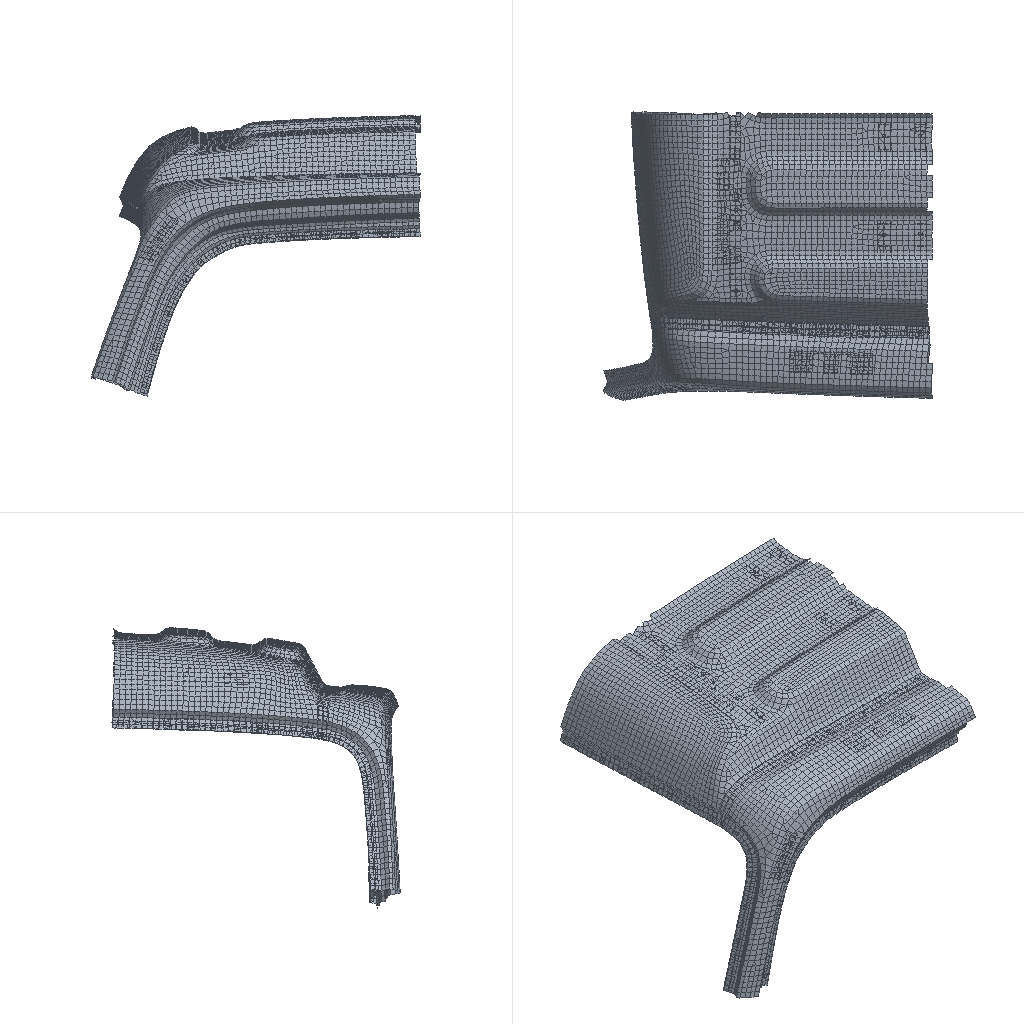Simulation study | nastran
Set-up summary:
category,name,step,type,value,unit,region
solver,nx_nastran
units,not stated in the deck,,not stated
analysis,deck,,static,static
analysis,solution,,SOL,101
load_step,SUBCASE 2,2,SUBCASE,SPC=2 LOAD=3
load_step,SUBCASE 3,3,SUBCASE,SPC=2 LOAD=4
load_step,SUBCASE 4,4,SUBCASE,SPC=2 LOAD=5
load_step,requested,,,3
mesh,nodes,,,9383
mesh,elements,,,8376
element_type,CHEXA,,unverified,79
element_type,CQUAD4,,shell,8105
element_type,CTRIA3,,shell,271
load,load commands in deck,,count,3
bc,support commands in deck,,count,307
check,setup vs results,,match,"every grid point's frame and coordinates and every element id; grid points of CHEXA, CQUAD4, CTRIA3 elements"
Nastran input file, long lists of numbers shortened:
$$------------------------------------------------------------------------------$
$$                                                                              $
$$ NASTRAN Input Deck Generated by HyperMesh Version  :10.0buil                 $
$$ Generated using HyperMesh-Nastran Template Version : 10.0build60
$$                                                                              $
$$   Template:  general                                                         $
$$                                                                              $
$$------------------------------------------------------------------------------$
$$------------------------------------------------------------------------------$
$$                      Executive Control Cards                                 $
$$------------------------------------------------------------------------------$
SOL 101
CEND
$$------------------------------------------------------------------------------$
$$                      Case Control Cards                                      $
$$------------------------------------------------------------------------------$
  DISPLACEMENT = ALL
  ESE = ALL
$
$HMNAME LOADSTEP               2"fx"
SUBCASE       2
  LABEL=  fx
  SPC =        2
  LOAD =        3
$
$HMNAME LOADSTEP               3"fy"
SUBCASE       3
  LABEL=  fy
  SPC =        2
  LOAD =        4
$
$HMNAME LOADSTEP               4"fz"
SUBCASE       4
  LABEL=  fz
  SPC =        2
  LOAD =        5
$$------------------------------------------------------------------------------$
$$                      Bulk Data Cards                                         $
$$------------------------------------------------------------------------------$
BEGIN BULK
PARAM,POST,-1
$$
$$  GRID Data
$$
GRID        7929        -566.911-803.2  1679.83
GRID        7931        -569.022-826.1571680.574
$ (9381 more lines like these left out)
$$
$$  SPOINT Data
$$
$$
$$------------------------------------------------------------------------------$
$$             Group Definitions                                                $
$$------------------------------------------------------------------------------$
$
$ RBE2 Elements - Single dependent node
$
RBE2     101299954027382  12345654025279
RBE2     101300054027422  12345654025448
RBE2     101300154027396  12345654025282
RBE2     101300254027434  12345654025455
$
$HMMOVE 84022688
$        1012999THRU     1013002
$
$$
$$ RBE2 Elements - Multiple dependent nodes
$$
RBE2     101299884098466  1234565401882054018821540188665401886754018928+
+       5401892954018963540190085401904654019085540190875401912054019121+
+       5401915754019158540192275401922854019232540193385401933954019340+
+       5401934554019347540193495401939554019396540194365401943854019477+
+       5401947854019522540195245402209754022124540221305402213654022778+
+       5402277954024651540252745402528054025281540252865402528754025350+
+       5402535454025372540253765402540054025407540254125402543054025466+
+       5402547954025489540254955402640354027322540274025402740854027423+
+
$
$HMMOVE 84022688
$        1012998
$
$
$  RBE3 Elements
$
RBE3      997760        84084287  1234560.347438     123540365920.132295+
+            123540365910.143473     123540365980.376794     12354036600
RBE3      997761        84084288  1234560.017003     123540365950.005887+
+            123540365930.251313     123540365910.725797     12354036592
$ (1036 more lines like these left out)
$
$HMMOVE 84022687
$         997760THRU      997763  997765THRU      997768  998048THRU      998051
$         998053THRU      998060  998062THRU      998069  998071THRU      998074
$ (29 more lines like these left out)
CTRIA3     28391       1540183315401833054017953
CTRIA3     28397       1540183345401833254018333
$ (269 more lines like these left out)
$
$HMMOVE 54001010
$          28391   28397   28681   28705   28725   39562THRU       39563  642518
$         642528  643114  643132  643135  643229  643294  643369  643386  643421
$ (58 more lines like these left out)
CQUAD4     27171       154017119540170245401702354017118
CQUAD4     27172       154017118540170235401702254017117
$ (8103 more lines like these left out)
$
$HMMOVE 54001010
$          27171THRU       27172   28222   28239   28245   28263   28265   28279
$          28290   28298   28312   28350   28358   28368THRU       28369   28380
$ (235 more lines like these left out)
CHEXA     990291      12   37175   37176   37177   371808405882884058833+
+       8405888684058812
CHEXA     990292      12   37180   37177   37178   371798405881284058886+
+       8405882484058820
$ (154 more lines like these left out)
$
$HMMOVE       16
$         990291THRU      990304
$
$ (84 more lines like these left out)
PSHELL         1       10.8            1               1
$
$HMNAME PROP                   2"120T" 4
$HWCOLOR PROP                  2       4
PSHELL         2       11.2            1               1
$
$HMNAME PROP                   9"70T" 4
$HWCOLOR PROP                  9      17
PSHELL         9       10.7            1               1
$$
$$  PSOLID Data
$
$HMNAME PROP                  12"glue" 5
$HWCOLOR PROP                 12      21
PSOLID        12       8
$
$HMNAME PROP                  15"spot" 5
$HWCOLOR PROP                 15      24
PSOLID        15       1
$$
$$------------------------------------------------------------------------------$
$$                      Material Definition Cards                               $
$$------------------------------------------------------------------------------$
$$--------------------------------------------------------------
$$ HYPERMESH TAGS
$$--------------------------------------------------------------
$$BEGIN TAGS
$$END TAGS
$$
$$  MAT1 Data
$
$HMNAME MAT                    1"steel" "MAT1"
$HWCOLOR MAT                   1       3
MAT1           1210000.0        0.3     7.90E-09
$
$HMNAME MAT                    8"glue" "MAT1"
$HWCOLOR MAT                   8       4
MAT1           8400.0           0.4     1.00E-10
$$
$$
$$
$$------------------------------------------------------------------------------$
$ (42 more lines like these left out)
SPC            2   37072  1234560.0
SPC            2   37172  1234560.0
SPC            2   37173  1234560.0
SPC            2   37174  1234560.0
$ (303 more lines like these left out)
$$
$$  FORCE Data
$$
FORCE          384098466       01.0     140.0   0.0     0.0
FORCE          484098466       01.0     0.0     320.0   0.0
FORCE          584098466       01.0     0.0     0.0     140.0
$HMASSEM 5400010       4 5400010
$HMASSEM_IDS    54001210540014105400101054003110540033105400531054005410
$HMASSEM 5700010       8 5700010
$HMASSEM_IDS    57001010570021105700221057003110      16
$
ENDDATA
Results summary:
result,analysis,,,static
result,last_loadstep,,,3
result,primary field,,,displacements
result,max displacement,,,3.059,model units